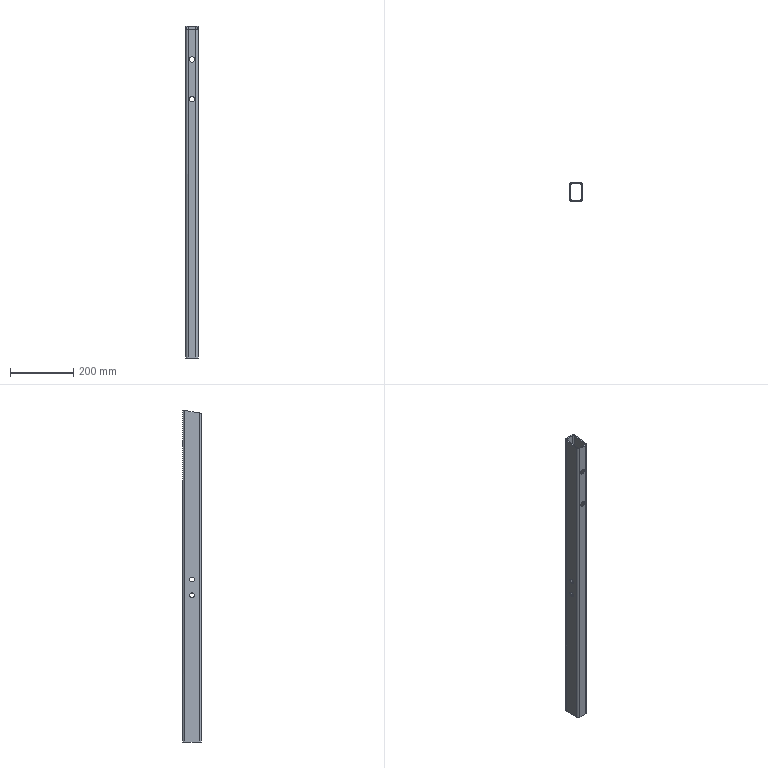Part | SolidWorks | features BaseBody 1 | 1 solid | 34 faces | box 40 x 60 x 1052 mm | volume 553157 mm3 | cylinder 24 | plane 10 | commonest cylinder face diameters 15 x12 17 x8 9 x4
STEP:
#1=CARTESIAN_POINT('',(-17.,7.5,465.));
#2=VERTEX_POINT('',#1);
#3=CARTESIAN_POINT('',(-17.,-7.5,465.));
#4=VERTEX_POINT('',#3);
#5=CARTESIAN_POINT('',(-17.,0.,465.));
#6=DIRECTION('',(-1.,0.,0.));
#7=DIRECTION('',(0.,-1.,0.));
#8=AXIS2_PLACEMENT_3D('',#5,#6,#7);
#9=CIRCLE('',#8,7.5);
#10=EDGE_CURVE('',#2,#4,#9,.T.);
#11=ORIENTED_EDGE('',*,*,#10,.F.);
#12=CARTESIAN_POINT('',(-20.,7.5,465.));
#13=VERTEX_POINT('',#12);
#14=CARTESIAN_POINT('',(1034.474,7.5,465.));
#15=DIRECTION('',(-1.,0.,0.));
#16=VECTOR('',#15,1000.);
#17=LINE('',#14,#16);
#18=EDGE_CURVE('',#2,#13,#17,.T.);
#19=ORIENTED_EDGE('',*,*,#18,.T.);
#20=CARTESIAN_POINT('',(-20.,-7.5,465.));
#21=VERTEX_POINT('',#20);
#22=CARTESIAN_POINT('',(-20.,0.,465.));
#23=DIRECTION('',(1.,0.,0.));
#24=DIRECTION('',(0.,-1.,0.));
#25=AXIS2_PLACEMENT_3D('',#22,#23,#24);
#26=CIRCLE('',#25,7.5);
#27=EDGE_CURVE('',#21,#13,#26,.T.);
#28=ORIENTED_EDGE('',*,*,#27,.F.);
#29=CARTESIAN_POINT('',(1034.474,-7.5,465.));
#30=DIRECTION('',(-1.,0.,0.));
#31=VECTOR('',#30,1000.);
#32=LINE('',#29,#31);
#33=EDGE_CURVE('',#4,#21,#32,.T.);
#34=ORIENTED_EDGE('',*,*,#33,.F.);
#35=EDGE_LOOP('',(#11,#19,#28,#34));
#36=FACE_OUTER_BOUND('',#35,.T.);
#37=CARTESIAN_POINT('',(1034.474,0.,465.));
#38=DIRECTION('',(-1.,0.,0.));
#39=DIRECTION('',(0.,-1.,0.));
#40=AXIS2_PLACEMENT_3D('',#37,#38,#39);
#41=CYLINDRICAL_SURFACE('',#40,7.5);
#42=ADVANCED_FACE('',(#36),#41,.F.);
#43=CARTESIAN_POINT('',(-17.,7.5,515.));
#44=VERTEX_POINT('',#43);
#45=CARTESIAN_POINT('',(-17.,-7.5,515.));
#46=VERTEX_POINT('',#45);
#47=CARTESIAN_POINT('',(-17.,0.,515.));
#48=DIRECTION('',(-1.,0.,0.));
#49=DIRECTION('',(0.,-1.,0.));
#50=AXIS2_PLACEMENT_3D('',#47,#48,#49);
#51=CIRCLE('',#50,7.5);
#52=EDGE_CURVE('',#44,#46,#51,.T.);
#53=ORIENTED_EDGE('',*,*,#52,.F.);
#54=CARTESIAN_POINT('',(-20.,7.5,515.));
#55=VERTEX_POINT('',#54);
#56=CARTESIAN_POINT('',(1034.474,7.5,515.));
#57=DIRECTION('',(-1.,0.,0.));
#58=VECTOR('',#57,1000.);
#59=LINE('',#56,#58);
#60=EDGE_CURVE('',#44,#55,#59,.T.);
#61=ORIENTED_EDGE('',*,*,#60,.T.);
#62=CARTESIAN_POINT('',(-20.,-7.5,515.));
#63=VERTEX_POINT('',#62);
#64=CARTESIAN_POINT('',(-20.,0.,515.));
#65=DIRECTION('',(1.,0.,0.));
#66=DIRECTION('',(0.,-1.,0.));
#67=AXIS2_PLACEMENT_3D('',#64,#65,#66);
#68=CIRCLE('',#67,7.5);
#69=EDGE_CURVE('',#63,#55,#68,.T.);
#70=ORIENTED_EDGE('',*,*,#69,.F.);
#71=CARTESIAN_POINT('',(1034.474,-7.5,515.));
#72=DIRECTION('',(-1.,0.,0.));
#73=VECTOR('',#72,1000.);
#74=LINE('',#71,#73);
#75=EDGE_CURVE('',#46,#63,#74,.T.);
#76=ORIENTED_EDGE('',*,*,#75,.F.);
#77=EDGE_LOOP('',(#53,#61,#70,#76));
#78=FACE_OUTER_BOUND('',#77,.T.);
#79=CARTESIAN_POINT('',(1034.474,0.,515.));
#80=DIRECTION('',(-1.,0.,0.));
#81=DIRECTION('',(0.,-1.,0.));
#82=AXIS2_PLACEMENT_3D('',#79,#80,#81);
#83=CYLINDRICAL_SURFACE('',#82,7.5);
#84=ADVANCED_FACE('',(#78),#83,.F.);
#85=CARTESIAN_POINT('',(0.,-30.,937.5));
#86=VERTEX_POINT('',#85);
#87=CARTESIAN_POINT('',(0.,-30.,954.5));
#88=VERTEX_POINT('',#87);
#89=CARTESIAN_POINT('',(0.,-30.,946.));
#90=DIRECTION('',(0.,1.,0.));
#91=DIRECTION('',(0.,0.,1.));
#92=AXIS2_PLACEMENT_3D('',#89,#90,#91);
#93=CIRCLE('',#92,8.5);
#94=EDGE_CURVE('',#86,#88,#93,.T.);
#95=ORIENTED_EDGE('',*,*,#94,.F.);
#96=CARTESIAN_POINT('',(0.,-27.,937.5));
#97=VERTEX_POINT('',#96);
#98=CARTESIAN_POINT('',(0.,-1024.474,937.5));
#99=DIRECTION('',(0.,1.,0.));
#100=VECTOR('',#99,1000.);
#101=LINE('',#98,#100);
#102=EDGE_CURVE('',#86,#97,#101,.T.);
#103=ORIENTED_EDGE('',*,*,#102,.T.);
#104=CARTESIAN_POINT('',(0.,-27.,954.5));
#105=VERTEX_POINT('',#104);
#106=CARTESIAN_POINT('',(0.,-27.,946.));
#107=DIRECTION('',(0.,1.,0.));
#108=DIRECTION('',(0.,0.,1.));
#109=AXIS2_PLACEMENT_3D('',#106,#107,#108);
#110=CIRCLE('',#109,8.5);
#111=EDGE_CURVE('',#97,#105,#110,.T.);
#112=ORIENTED_EDGE('',*,*,#111,.T.);
#113=CARTESIAN_POINT('',(0.,-1024.474,954.5));
#114=DIRECTION('',(0.,1.,0.));
#115=VECTOR('',#114,1000.);
#116=LINE('',#113,#115);
#117=EDGE_CURVE('',#88,#105,#116,.T.);
#118=ORIENTED_EDGE('',*,*,#117,.F.);
#119=EDGE_LOOP('',(#95,#103,#112,#118));
#120=FACE_OUTER_BOUND('',#119,.T.);
#121=CARTESIAN_POINT('',(0.,-1024.474,946.));
#122=DIRECTION('',(0.,1.,0.));
#123=DIRECTION('',(0.,0.,1.));
#124=AXIS2_PLACEMENT_3D('',#121,#122,#123);
#125=CYLINDRICAL_SURFACE('',#124,8.5);
#126=ADVANCED_FACE('',(#120),#125,.F.);
#127=CARTESIAN_POINT('',(0.,-30.,811.5));
#128=VERTEX_POINT('',#127);
#129=CARTESIAN_POINT('',(0.,-30.,828.5));
#130=VERTEX_POINT('',#129);
#131=CARTESIAN_POINT('',(0.,-30.,820.));
#132=DIRECTION('',(0.,1.,0.));
#133=DIRECTION('',(0.,0.,1.));
#134=AXIS2_PLACEMENT_3D('',#131,#132,#133);
#135=CIRCLE('',#134,8.5);
#136=EDGE_CURVE('',#128,#130,#135,.T.);
#137=ORIENTED_EDGE('',*,*,#136,.F.);
#138=CARTESIAN_POINT('',(0.,-27.,811.5));
#139=VERTEX_POINT('',#138);
#140=CARTESIAN_POINT('',(0.,-1024.474,811.5));
#141=DIRECTION('',(0.,1.,0.));
#142=VECTOR('',#141,1000.);
#143=LINE('',#140,#142);
#144=EDGE_CURVE('',#128,#139,#143,.T.);
#145=ORIENTED_EDGE('',*,*,#144,.T.);
#146=CARTESIAN_POINT('',(0.,-27.,828.5));
#147=VERTEX_POINT('',#146);
#148=CARTESIAN_POINT('',(0.,-27.,820.));
#149=DIRECTION('',(0.,1.,0.));
#150=DIRECTION('',(0.,0.,1.));
#151=AXIS2_PLACEMENT_3D('',#148,#149,#150);
#152=CIRCLE('',#151,8.5);
#153=EDGE_CURVE('',#139,#147,#152,.T.);
#154=ORIENTED_EDGE('',*,*,#153,.T.);
#155=CARTESIAN_POINT('',(0.,-1024.474,828.5));
#156=DIRECTION('',(0.,1.,0.));
#157=VECTOR('',#156,1000.);
#158=LINE('',#155,#157);
#159=EDGE_CURVE('',#130,#147,#158,.T.);
#160=ORIENTED_EDGE('',*,*,#159,.F.);
#161=EDGE_LOOP('',(#137,#145,#154,#160));
#162=FACE_OUTER_BOUND('',#161,.T.);
#163=CARTESIAN_POINT('',(0.,-1024.474,820.));
#164=DIRECTION('',(0.,1.,0.));
#165=DIRECTION('',(0.,0.,1.));
#166=AXIS2_PLACEMENT_3D('',#163,#164,#165);
#167=CYLINDRICAL_SURFACE('',#166,8.5);
#168=ADVANCED_FACE('',(#162),#167,.F.);
#169=CARTESIAN_POINT('',(0.,27.,954.5));
#170=VERTEX_POINT('',#169);
#171=CARTESIAN_POINT('',(0.,27.,937.5));
#172=VERTEX_POINT('',#171);
#173=CARTESIAN_POINT('',(0.,27.,946.));
#174=DIRECTION('',(0.,-1.,0.));
#175=DIRECTION('',(0.,0.,1.));
#176=AXIS2_PLACEMENT_3D('',#173,#174,#175);
#177=CIRCLE('',#176,8.5);
#178=EDGE_CURVE('',#170,#172,#177,.T.);
#179=ORIENTED_EDGE('',*,*,#178,.T.);
#180=CARTESIAN_POINT('',(0.,30.,937.5));
#181=VERTEX_POINT('',#180);
#182=CARTESIAN_POINT('',(0.,-1024.474,937.5));
#183=DIRECTION('',(0.,1.,0.));
#184=VECTOR('',#183,1000.);
#185=LINE('',#182,#184);
#186=EDGE_CURVE('',#172,#181,#185,.T.);
#187=ORIENTED_EDGE('',*,*,#186,.T.);
#188=CARTESIAN_POINT('',(0.,30.,954.5));
#189=VERTEX_POINT('',#188);
#190=CARTESIAN_POINT('',(0.,30.,946.));
#191=DIRECTION('',(0.,-1.,0.));
#192=DIRECTION('',(0.,0.,1.));
#193=AXIS2_PLACEMENT_3D('',#190,#191,#192);
#194=CIRCLE('',#193,8.5);
#195=EDGE_CURVE('',#189,#181,#194,.T.);
#196=ORIENTED_EDGE('',*,*,#195,.F.);
#197=CARTESIAN_POINT('',(0.,-1024.474,954.5));
#198=DIRECTION('',(0.,1.,0.));
#199=VECTOR('',#198,1000.);
#200=LINE('',#197,#199);
#201=EDGE_CURVE('',#170,#189,#200,.T.);
#202=ORIENTED_EDGE('',*,*,#201,.F.);
#203=EDGE_LOOP('',(#179,#187,#196,#202));
#204=FACE_OUTER_BOUND('',#203,.T.);
#205=CARTESIAN_POINT('',(0.,-1024.474,946.));
#206=DIRECTION('',(0.,1.,0.));
#207=DIRECTION('',(0.,0.,1.));
#208=AXIS2_PLACEMENT_3D('',#205,#206,#207);
#209=CYLINDRICAL_SURFACE('',#208,8.5);
#210=ADVANCED_FACE('',(#204),#209,.F.);
#211=CARTESIAN_POINT('',(0.,27.,828.5));
#212=VERTEX_POINT('',#211);
#213=CARTESIAN_POINT('',(0.,27.,811.5));
#214=VERTEX_POINT('',#213);
#215=CARTESIAN_POINT('',(0.,27.,820.));
#216=DIRECTION('',(0.,-1.,0.));
#217=DIRECTION('',(0.,0.,1.));
#218=AXIS2_PLACEMENT_3D('',#215,#216,#217);
#219=CIRCLE('',#218,8.5);
#220=EDGE_CURVE('',#212,#214,#219,.T.);
#221=ORIENTED_EDGE('',*,*,#220,.T.);
#222=CARTESIAN_POINT('',(0.,30.,811.5));
#223=VERTEX_POINT('',#222);
#224=CARTESIAN_POINT('',(0.,-1024.474,811.5));
#225=DIRECTION('',(0.,1.,0.));
#226=VECTOR('',#225,1000.);
#227=LINE('',#224,#226);
#228=EDGE_CURVE('',#214,#223,#227,.T.);
#229=ORIENTED_EDGE('',*,*,#228,.T.);
#230=CARTESIAN_POINT('',(0.,30.,828.5));
#231=VERTEX_POINT('',#230);
#232=CARTESIAN_POINT('',(0.,30.,820.));
#233=DIRECTION('',(0.,-1.,0.));
#234=DIRECTION('',(0.,0.,1.));
#235=AXIS2_PLACEMENT_3D('',#232,#233,#234);
#236=CIRCLE('',#235,8.5);
#237=EDGE_CURVE('',#231,#223,#236,.T.);
#238=ORIENTED_EDGE('',*,*,#237,.F.);
#239=CARTESIAN_POINT('',(0.,-1024.474,828.5));
#240=DIRECTION('',(0.,1.,0.));
#241=VECTOR('',#240,1000.);
#242=LINE('',#239,#241);
#243=EDGE_CURVE('',#212,#231,#242,.T.);
#244=ORIENTED_EDGE('',*,*,#243,.F.);
#245=EDGE_LOOP('',(#221,#229,#238,#244));
#246=FACE_OUTER_BOUND('',#245,.T.);
#247=CARTESIAN_POINT('',(0.,-1024.474,820.));
#248=DIRECTION('',(0.,1.,0.));
#249=DIRECTION('',(0.,0.,1.));
#250=AXIS2_PLACEMENT_3D('',#247,#248,#249);
#251=CYLINDRICAL_SURFACE('',#250,8.5);
#252=ADVANCED_FACE('',(#246),#251,.F.);
#253=CARTESIAN_POINT('',(20.,7.5,465.));
#254=VERTEX_POINT('',#253);
#255=CARTESIAN_POINT('',(20.,-7.5,465.));
#256=VERTEX_POINT('',#255);
#257=CARTESIAN_POINT('',(20.,0.,465.));
#258=DIRECTION('',(-1.,0.,0.));
#259=DIRECTION('',(0.,-1.,0.));
#260=AXIS2_PLACEMENT_3D('',#257,#258,#259);
#261=CIRCLE('',#260,7.5);
#262=EDGE_CURVE('',#254,#256,#261,.T.);
#263=ORIENTED_EDGE('',*,*,#262,.F.);
#264=CARTESIAN_POINT('',(17.,7.5,465.));
#265=VERTEX_POINT('',#264);
#266=CARTESIAN_POINT('',(1034.474,7.5,465.));
#267=DIRECTION('',(-1.,0.,0.));
#268=VECTOR('',#267,1000.);
#269=LINE('',#266,#268);
#270=EDGE_CURVE('',#254,#265,#269,.T.);
#271=ORIENTED_EDGE('',*,*,#270,.T.);
#272=CARTESIAN_POINT('',(17.,-7.5,465.));
#273=VERTEX_POINT('',#272);
#274=CARTESIAN_POINT('',(17.,0.,465.));
#275=DIRECTION('',(-1.,0.,0.));
#276=DIRECTION('',(0.,-1.,0.));
#277=AXIS2_PLACEMENT_3D('',#274,#275,#276);
#278=CIRCLE('',#277,7.5);
#279=EDGE_CURVE('',#265,#273,#278,.T.);
#280=ORIENTED_EDGE('',*,*,#279,.T.);
#281=CARTESIAN_POINT('',(1034.474,-7.5,465.));
#282=DIRECTION('',(-1.,0.,0.));
#283=VECTOR('',#282,1000.);
#284=LINE('',#281,#283);
#285=EDGE_CURVE('',#256,#273,#284,.T.);
#286=ORIENTED_EDGE('',*,*,#285,.F.);
#287=EDGE_LOOP('',(#263,#271,#280,#286));
#288=FACE_OUTER_BOUND('',#287,.T.);
#289=CARTESIAN_POINT('',(1034.474,0.,465.));
#290=DIRECTION('',(-1.,0.,0.));
#291=DIRECTION('',(0.,-1.,0.));
#292=AXIS2_PLACEMENT_3D('',#289,#290,#291);
#293=CYLINDRICAL_SURFACE('',#292,7.5);
#294=ADVANCED_FACE('',(#288),#293,.F.);
#295=CARTESIAN_POINT('',(20.,7.5,515.));
#296=VERTEX_POINT('',#295);
#297=CARTESIAN_POINT('',(20.,-7.5,515.));
#298=VERTEX_POINT('',#297);
#299=CARTESIAN_POINT('',(20.,0.,515.));
#300=DIRECTION('',(-1.,0.,0.));
#301=DIRECTION('',(0.,-1.,0.));
#302=AXIS2_PLACEMENT_3D('',#299,#300,#301);
#303=CIRCLE('',#302,7.5);
#304=EDGE_CURVE('',#296,#298,#303,.T.);
#305=ORIENTED_EDGE('',*,*,#304,.F.);
#306=CARTESIAN_POINT('',(17.,7.5,515.));
#307=VERTEX_POINT('',#306);
#308=CARTESIAN_POINT('',(1034.474,7.5,515.));
#309=DIRECTION('',(-1.,0.,0.));
#310=VECTOR('',#309,1000.);
#311=LINE('',#308,#310);
#312=EDGE_CURVE('',#296,#307,#311,.T.);
#313=ORIENTED_EDGE('',*,*,#312,.T.);
#314=CARTESIAN_POINT('',(17.,-7.5,515.));
#315=VERTEX_POINT('',#314);
#316=CARTESIAN_POINT('',(17.,0.,515.));
#317=DIRECTION('',(-1.,0.,0.));
#318=DIRECTION('',(0.,-1.,0.));
#319=AXIS2_PLACEMENT_3D('',#316,#317,#318);
#320=CIRCLE('',#319,7.5);
#321=EDGE_CURVE('',#307,#315,#320,.T.);
#322=ORIENTED_EDGE('',*,*,#321,.T.);
#323=CARTESIAN_POINT('',(1034.474,-7.5,515.));
#324=DIRECTION('',(-1.,0.,0.));
#325=VECTOR('',#324,1000.);
#326=LINE('',#323,#325);
#327=EDGE_CURVE('',#298,#315,#326,.T.);
#328=ORIENTED_EDGE('',*,*,#327,.F.);
#329=EDGE_LOOP('',(#305,#313,#322,#328));
#330=FACE_OUTER_BOUND('',#329,.T.);
#331=CARTESIAN_POINT('',(1034.474,0.,515.));
#332=DIRECTION('',(-1.,0.,0.));
#333=DIRECTION('',(0.,-1.,0.));
#334=AXIS2_PLACEMENT_3D('',#331,#332,#333);
#335=CYLINDRICAL_SURFACE('',#334,7.5);
#336=ADVANCED_FACE('',(#330),#335,.F.);
#337=ORIENTED_EDGE('',*,*,#27,.T.);
#338=CARTESIAN_POINT('',(-20.,0.,465.));
#339=DIRECTION('',(1.,0.,0.));
#340=DIRECTION('',(0.,-1.,0.));
#341=AXIS2_PLACEMENT_3D('',#338,#339,#340);
#342=CIRCLE('',#341,7.5);
#343=EDGE_CURVE('',#13,#21,#342,.T.);
#344=ORIENTED_EDGE('',*,*,#343,.T.);
#345=EDGE_LOOP('',(#337,#344));
#346=FACE_BOUND('',#345,.T.);
#347=ORIENTED_EDGE('',*,*,#69,.T.);
#348=CARTESIAN_POINT('',(-20.,0.,515.));
#349=DIRECTION('',(1.,0.,0.));
#350=DIRECTION('',(0.,-1.,0.));
#351=AXIS2_PLACEMENT_3D('',#348,#349,#350);
#352=CIRCLE('',#351,7.5);
#353=EDGE_CURVE('',#55,#63,#352,.T.);
#354=ORIENTED_EDGE('',*,*,#353,.T.);
#355=EDGE_LOOP('',(#347,#354));
#356=FACE_BOUND('',#355,.T.);
#357=CARTESIAN_POINT('',(-20.,22.5,0.));
#358=VERTEX_POINT('',#357);
#359=CARTESIAN_POINT('',(-20.,-22.5,0.));
#360=VERTEX_POINT('',#359);
#361=CARTESIAN_POINT('',(-20.,-22.5,0.));
#362=DIRECTION('',(0.,-1.,0.));
#363=VECTOR('',#362,1000.);
#364=LINE('',#361,#363);
#365=EDGE_CURVE('',#358,#360,#364,.T.);
#366=ORIENTED_EDGE('',*,*,#365,.T.);
#367=CARTESIAN_POINT('',(-20.,-22.5,1042.748));
#368=VERTEX_POINT('',#367);
#369=CARTESIAN_POINT('',(-20.,-22.5,0.));
#370=DIRECTION('',(0.,0.,1.));
#371=VECTOR('',#370,1000.);
#372=LINE('',#369,#371);
#373=EDGE_CURVE('',#360,#368,#372,.T.);
#374=ORIENTED_EDGE('',*,*,#373,.T.);
#375=CARTESIAN_POINT('',(-20.,22.5,1050.683));
#376=VERTEX_POINT('',#375);
#377=CARTESIAN_POINT('',(-20.,-22.5,1042.748));
#378=DIRECTION('',(0.,0.9848,0.1736));
#379=VECTOR('',#378,1000.);
#380=LINE('',#377,#379);
#381=EDGE_CURVE('',#368,#376,#380,.T.);
#382=ORIENTED_EDGE('',*,*,#381,.T.);
#383=CARTESIAN_POINT('',(-20.,22.5,0.));
#384=DIRECTION('',(0.,0.,-1.));
#385=VECTOR('',#384,1000.);
#386=LINE('',#383,#385);
#387=EDGE_CURVE('',#376,#358,#386,.T.);
#388=ORIENTED_EDGE('',*,*,#387,.T.);
#389=EDGE_LOOP('',(#366,#374,#382,#388));
#390=FACE_OUTER_BOUND('',#389,.T.);
#391=CARTESIAN_POINT('',(-20.,-22.5,0.));
#392=DIRECTION('',(-1.,0.,0.));
#393=DIRECTION('',(0.,-1.,0.));
#394=AXIS2_PLACEMENT_3D('',#391,#392,#393);
#395=PLANE('',#394);
#396=ADVANCED_FACE('',(#346,#356,#390),#395,.T.);
#397=ORIENTED_EDGE('',*,*,#18,.F.);
#398=CARTESIAN_POINT('',(-17.,0.,465.));
#399=DIRECTION('',(-1.,0.,0.));
#400=DIRECTION('',(0.,-1.,0.));
#401=AXIS2_PLACEMENT_3D('',#398,#399,#400);
#402=CIRCLE('',#401,7.5);
#403=EDGE_CURVE('',#4,#2,#402,.T.);
#404=ORIENTED_EDGE('',*,*,#403,.F.);
#405=ORIENTED_EDGE('',*,*,#33,.T.);
#406=ORIENTED_EDGE('',*,*,#343,.F.);
#407=EDGE_LOOP('',(#397,#404,#405,#406));
#408=FACE_OUTER_BOUND('',#407,.T.);
#409=CARTESIAN_POINT('',(1034.474,0.,465.));
#410=DIRECTION('',(-1.,0.,0.));
#411=DIRECTION('',(0.,-1.,0.));
#412=AXIS2_PLACEMENT_3D('',#409,#410,#411);
#413=CYLINDRICAL_SURFACE('',#412,7.5);
#414=ADVANCED_FACE('',(#408),#413,.F.);
#415=ORIENTED_EDGE('',*,*,#60,.F.);
#416=CARTESIAN_POINT('',(-17.,0.,515.));
#417=DIRECTION('',(-1.,0.,0.));
#418=DIRECTION('',(0.,-1.,0.));
#419=AXIS2_PLACEMENT_3D('',#416,#417,#418);
#420=CIRCLE('',#419,7.5);
#421=EDGE_CURVE('',#46,#44,#420,.T.);
#422=ORIENTED_EDGE('',*,*,#421,.F.);
#423=ORIENTED_EDGE('',*,*,#75,.T.);
#424=ORIENTED_EDGE('',*,*,#353,.F.);
#425=EDGE_LOOP('',(#415,#422,#423,#424));
#426=FACE_OUTER_BOUND('',#425,.T.);
#427=CARTESIAN_POINT('',(1034.474,0.,515.));
#428=DIRECTION('',(-1.,0.,0.));
#429=DIRECTION('',(0.,-1.,0.));
#430=AXIS2_PLACEMENT_3D('',#427,#428,#429);
#431=CYLINDRICAL_SURFACE('',#430,7.5);
#432=ADVANCED_FACE('',(#426),#431,.F.);
#433=CARTESIAN_POINT('',(-12.5,-30.,0.));
#434=VERTEX_POINT('',#433);
#435=CARTESIAN_POINT('',(-12.5,-22.5,0.));
#436=DIRECTION('',(0.,0.,1.));
#437=DIRECTION('',(1.,0.,0.));
#438=AXIS2_PLACEMENT_3D('',#435,#436,#437);
#439=CIRCLE('',#438,7.5);
#440=EDGE_CURVE('',#360,#434,#439,.T.);
#441=ORIENTED_EDGE('',*,*,#440,.T.);
#442=CARTESIAN_POINT('',(-12.5,-30.,1041.426));
#443=VERTEX_POINT('',#442);
#444=CARTESIAN_POINT('',(-12.5,-30.,0.));
#445=DIRECTION('',(0.,0.,1.));
#446=VECTOR('',#445,1000.);
#447=LINE('',#444,#446);
#448=EDGE_CURVE('',#434,#443,#447,.T.);
#449=ORIENTED_EDGE('',*,*,#448,.T.);
#450=CARTESIAN_POINT('',(-12.5,-30.,1041.426));
#451=CARTESIAN_POINT('',(-16.893,-30.,1041.426));
#452=CARTESIAN_POINT('',(-20.,-26.893,1041.974));
#453=CARTESIAN_POINT('',(-20.,-22.5,1042.748));
#454=(BOUNDED_CURVE()B_SPLINE_CURVE(3,(#450,#451,#452,#453),.UNSPECIFIED.,.F.,.T.)B_SPLINE_CURVE_WITH_KNOTS((4,4),(3.142,4.712),.UNSPECIFIED.)CURVE()GEOMETRIC_REPRESENTATION_ITEM()RATIONAL_B_SPLINE_CURVE((1.,0.8047,0.8047,1.))REPRESENTATION_ITEM(''));
#455=EDGE_CURVE('',#443,#368,#454,.T.);
#456=ORIENTED_EDGE('',*,*,#455,.T.);
#457=ORIENTED_EDGE('',*,*,#373,.F.);
#458=EDGE_LOOP('',(#441,#449,#456,#457));
#459=FACE_OUTER_BOUND('',#458,.T.);
#460=CARTESIAN_POINT('',(-12.5,-22.5,0.));
#461=DIRECTION('',(0.,0.,1.));
#462=DIRECTION('',(1.,0.,0.));
#463=AXIS2_PLACEMENT_3D('',#460,#461,#462);
#464=CYLINDRICAL_SURFACE('',#463,7.5);
#465=ADVANCED_FACE('',(#459),#464,.T.);
#466=CARTESIAN_POINT('',(-17.,22.5,0.));
#467=VERTEX_POINT('',#466);
#468=CARTESIAN_POINT('',(-12.5,27.,0.));
#469=VERTEX_POINT('',#468);
#470=CARTESIAN_POINT('',(-12.5,22.5,0.));
#471=DIRECTION('',(0.,0.,-1.));
#472=DIRECTION('',(1.,0.,0.));
#473=AXIS2_PLACEMENT_3D('',#470,#471,#472);
#474=CIRCLE('',#473,4.5);
#475=EDGE_CURVE('',#467,#469,#474,.T.);
#476=ORIENTED_EDGE('',*,*,#475,.F.);
#477=CARTESIAN_POINT('',(-17.,-22.5,0.));
#478=VERTEX_POINT('',#477);
#479=CARTESIAN_POINT('',(-17.,0.,0.));
#480=DIRECTION('',(0.,1.,0.));
#481=VECTOR('',#480,1000.);
#482=LINE('',#479,#481);
#483=EDGE_CURVE('',#478,#467,#482,.T.);
#484=ORIENTED_EDGE('',*,*,#483,.F.);
#485=CARTESIAN_POINT('',(-12.5,-27.,0.));
#486=VERTEX_POINT('',#485);
#487=CARTESIAN_POINT('',(-12.5,-22.5,0.));
#488=DIRECTION('',(0.,0.,-1.));
#489=DIRECTION('',(1.,0.,0.));
#490=AXIS2_PLACEMENT_3D('',#487,#488,#489);
#491=CIRCLE('',#490,4.5);
#492=EDGE_CURVE('',#486,#478,#491,.T.);
#493=ORIENTED_EDGE('',*,*,#492,.F.);
#494=CARTESIAN_POINT('',(12.5,-27.,0.));
#495=VERTEX_POINT('',#494);
#496=CARTESIAN_POINT('',(0.,-27.,0.));
#497=DIRECTION('',(-1.,0.,0.));
#498=VECTOR('',#497,1000.);
#499=LINE('',#496,#498);
#500=EDGE_CURVE('',#495,#486,#499,.T.);
#501=ORIENTED_EDGE('',*,*,#500,.F.);
#502=CARTESIAN_POINT('',(17.,-22.5,0.));
#503=VERTEX_POINT('',#502);
#504=CARTESIAN_POINT('',(12.5,-22.5,0.));
#505=DIRECTION('',(0.,0.,-1.));
#506=DIRECTION('',(1.,0.,0.));
#507=AXIS2_PLACEMENT_3D('',#504,#505,#506);
#508=CIRCLE('',#507,4.5);
#509=EDGE_CURVE('',#503,#495,#508,.T.);
#510=ORIENTED_EDGE('',*,*,#509,.F.);
#511=CARTESIAN_POINT('',(17.,22.5,0.));
#512=VERTEX_POINT('',#511);
#513=CARTESIAN_POINT('',(17.,0.,0.));
#514=DIRECTION('',(0.,-1.,0.));
#515=VECTOR('',#514,1000.);
#516=LINE('',#513,#515);
#517=EDGE_CURVE('',#512,#503,#516,.T.);
#518=ORIENTED_EDGE('',*,*,#517,.F.);
#519=CARTESIAN_POINT('',(12.5,27.,0.));
#520=VERTEX_POINT('',#519);
#521=CARTESIAN_POINT('',(12.5,22.5,0.));
#522=DIRECTION('',(0.,0.,-1.));
#523=DIRECTION('',(1.,0.,0.));
#524=AXIS2_PLACEMENT_3D('',#521,#522,#523);
#525=CIRCLE('',#524,4.5);
#526=EDGE_CURVE('',#520,#512,#525,.T.);
#527=ORIENTED_EDGE('',*,*,#526,.F.);
#528=CARTESIAN_POINT('',(0.,27.,0.));
#529=DIRECTION('',(1.,0.,0.));
#530=VECTOR('',#529,1000.);
#531=LINE('',#528,#530);
#532=EDGE_CURVE('',#469,#520,#531,.T.);
#533=ORIENTED_EDGE('',*,*,#532,.F.);
#534=EDGE_LOOP('',(#476,#484,#493,#501,#510,#518,#527,#533));
#535=FACE_BOUND('',#534,.T.);
#536=CARTESIAN_POINT('',(-12.5,30.,0.));
#537=VERTEX_POINT('',#536);
#538=CARTESIAN_POINT('',(-12.5,22.5,0.));
#539=DIRECTION('',(0.,0.,1.));
#540=DIRECTION('',(1.,0.,0.));
#541=AXIS2_PLACEMENT_3D('',#538,#539,#540);
#542=CIRCLE('',#541,7.5);
#543=EDGE_CURVE('',#537,#358,#542,.T.);
#544=ORIENTED_EDGE('',*,*,#543,.F.);
#545=CARTESIAN_POINT('',(12.5,30.,0.));
#546=VERTEX_POINT('',#545);
#547=CARTESIAN_POINT('',(0.,30.,0.));
#548=DIRECTION('',(-1.,0.,0.));
#549=VECTOR('',#548,1000.);
#550=LINE('',#547,#549);
#551=EDGE_CURVE('',#546,#537,#550,.T.);
#552=ORIENTED_EDGE('',*,*,#551,.F.);
#553=CARTESIAN_POINT('',(20.,22.5,0.));
#554=VERTEX_POINT('',#553);
#555=CARTESIAN_POINT('',(12.5,22.5,0.));
#556=DIRECTION('',(0.,0.,1.));
#557=DIRECTION('',(1.,0.,0.));
#558=AXIS2_PLACEMENT_3D('',#555,#556,#557);
#559=CIRCLE('',#558,7.5);
#560=EDGE_CURVE('',#554,#546,#559,.T.);
#561=ORIENTED_EDGE('',*,*,#560,.F.);
#562=CARTESIAN_POINT('',(20.,-22.5,0.));
#563=VERTEX_POINT('',#562);
#564=CARTESIAN_POINT('',(20.,0.,0.));
#565=DIRECTION('',(0.,1.,0.));
#566=VECTOR('',#565,1000.);
#567=LINE('',#564,#566);
#568=EDGE_CURVE('',#563,#554,#567,.T.);
#569=ORIENTED_EDGE('',*,*,#568,.F.);
#570=CARTESIAN_POINT('',(12.5,-30.,0.));
#571=VERTEX_POINT('',#570);
#572=CARTESIAN_POINT('',(12.5,-22.5,0.));
#573=DIRECTION('',(0.,0.,1.));
#574=DIRECTION('',(1.,0.,0.));
#575=AXIS2_PLACEMENT_3D('',#572,#573,#574);
#576=CIRCLE('',#575,7.5);
#577=EDGE_CURVE('',#571,#563,#576,.T.);
#578=ORIENTED_EDGE('',*,*,#577,.F.);
#579=CARTESIAN_POINT('',(0.,-30.,0.));
#580=DIRECTION('',(1.,0.,0.));
#581=VECTOR('',#580,1000.);
#582=LINE('',#579,#581);
#583=EDGE_CURVE('',#434,#571,#582,.T.);
#584=ORIENTED_EDGE('',*,*,#583,.F.);
#585=ORIENTED_EDGE('',*,*,#440,.F.);
#586=ORIENTED_EDGE('',*,*,#365,.F.);
#587=EDGE_LOOP('',(#544,#552,#561,#569,#578,#584,#585,#586));
#588=FACE_OUTER_BOUND('',#587,.T.);
#589=CARTESIAN_POINT('',(0.,0.,0.));
#590=DIRECTION('',(0.,0.,1.));
#591=DIRECTION('',(1.,0.,0.));
#592=AXIS2_PLACEMENT_3D('',#589,#590,#591);
#593=PLANE('',#592);
#594=ADVANCED_FACE('',(#535,#588),#593,.F.);
#595=ORIENTED_EDGE('',*,*,#543,.T.);
#596=ORIENTED_EDGE('',*,*,#387,.F.);
#597=CARTESIAN_POINT('',(-12.5,30.,1052.005));
#598=VERTEX_POINT('',#597);
#599=CARTESIAN_POINT('',(-20.,22.5,1050.683));
#600=CARTESIAN_POINT('',(-20.,26.893,1051.458));
#601=CARTESIAN_POINT('',(-16.893,30.,1052.005));
#602=CARTESIAN_POINT('',(-12.5,30.,1052.005));
#603=(BOUNDED_CURVE()B_SPLINE_CURVE(3,(#599,#600,#601,#602),.UNSPECIFIED.,.F.,.F.)B_SPLINE_CURVE_WITH_KNOTS((4,4),(4.712,6.283),.UNSPECIFIED.)CURVE()GEOMETRIC_REPRESENTATION_ITEM()RATIONAL_B_SPLINE_CURVE((1.,0.8047,0.8047,1.))REPRESENTATION_ITEM(''));
#604=EDGE_CURVE('',#376,#598,#603,.T.);
#605=ORIENTED_EDGE('',*,*,#604,.T.);
#606=CARTESIAN_POINT('',(-12.5,30.,0.));
#607=DIRECTION('',(0.,0.,-1.));
#608=VECTOR('',#607,1000.);
#609=LINE('',#606,#608);
#610=EDGE_CURVE('',#598,#537,#609,.T.);
#611=ORIENTED_EDGE('',*,*,#610,.T.);
#612=EDGE_LOOP('',(#595,#596,#605,#611));
#613=FACE_OUTER_BOUND('',#612,.T.);
#614=CARTESIAN_POINT('',(-12.5,22.5,0.));
#615=DIRECTION('',(0.,0.,1.));
#616=DIRECTION('',(1.,0.,0.));
#617=AXIS2_PLACEMENT_3D('',#614,#615,#616);
#618=CYLINDRICAL_SURFACE('',#617,7.5);
#619=ADVANCED_FACE('',(#613),#618,.T.);
#620=CARTESIAN_POINT('',(-17.,-22.5,1042.748));
#621=VERTEX_POINT('',#620);
#622=CARTESIAN_POINT('',(-12.5,-27.,1041.955));
#623=VERTEX_POINT('',#622);
#624=CARTESIAN_POINT('',(-17.,-22.5,1042.748));
#625=CARTESIAN_POINT('',(-17.,-25.136,1042.283));
#626=CARTESIAN_POINT('',(-15.136,-27.,1041.955));
#627=CARTESIAN_POINT('',(-12.5,-27.,1041.955));
#628=(BOUNDED_CURVE()B_SPLINE_CURVE(3,(#624,#625,#626,#627),.UNSPECIFIED.,.F.,.F.)B_SPLINE_CURVE_WITH_KNOTS((4,4),(1.571,3.142),.UNSPECIFIED.)CURVE()GEOMETRIC_REPRESENTATION_ITEM()RATIONAL_B_SPLINE_CURVE((1.,0.8047,0.8047,1.))REPRESENTATION_ITEM(''));
#629=EDGE_CURVE('',#621,#623,#628,.T.);
#630=ORIENTED_EDGE('',*,*,#629,.F.);
#631=CARTESIAN_POINT('',(-17.,22.5,1050.683));
#632=VERTEX_POINT('',#631);
#633=CARTESIAN_POINT('',(-17.,-178.999,1015.153));
#634=DIRECTION('',(0.,-0.9848,-0.1736));
#635=VECTOR('',#634,1000.);
#636=LINE('',#633,#635);
#637=EDGE_CURVE('',#632,#621,#636,.T.);
#638=ORIENTED_EDGE('',*,*,#637,.F.);
#639=CARTESIAN_POINT('',(-12.5,27.,1051.476));
#640=VERTEX_POINT('',#639);
#641=CARTESIAN_POINT('',(-12.5,27.,1051.476));
#642=CARTESIAN_POINT('',(-15.136,27.,1051.476));
#643=CARTESIAN_POINT('',(-17.,25.136,1051.148));
#644=CARTESIAN_POINT('',(-17.,22.5,1050.683));
#645=(BOUNDED_CURVE()B_SPLINE_CURVE(3,(#641,#642,#643,#644),.UNSPECIFIED.,.F.,.F.)B_SPLINE_CURVE_WITH_KNOTS((4,4),(0.,1.571),.UNSPECIFIED.)CURVE()GEOMETRIC_REPRESENTATION_ITEM()RATIONAL_B_SPLINE_CURVE((1.,0.8047,0.8047,1.))REPRESENTATION_ITEM(''));
#646=EDGE_CURVE('',#640,#632,#645,.T.);
#647=ORIENTED_EDGE('',*,*,#646,.F.);
#648=CARTESIAN_POINT('',(12.5,27.,1051.476));
#649=VERTEX_POINT('',#648);
#650=CARTESIAN_POINT('',(0.,27.,1051.476));
#651=DIRECTION('',(-1.,0.,0.));
#652=VECTOR('',#651,1000.);
#653=LINE('',#650,#652);
#654=EDGE_CURVE('',#649,#640,#653,.T.);
#655=ORIENTED_EDGE('',*,*,#654,.F.);
#656=CARTESIAN_POINT('',(17.,22.5,1050.683));
#657=VERTEX_POINT('',#656);
#658=CARTESIAN_POINT('',(17.,22.5,1050.683));
#659=CARTESIAN_POINT('',(17.,25.136,1051.148));
#660=CARTESIAN_POINT('',(15.136,27.,1051.476));
#661=CARTESIAN_POINT('',(12.5,27.,1051.476));
#662=(BOUNDED_CURVE()B_SPLINE_CURVE(3,(#658,#659,#660,#661),.UNSPECIFIED.,.F.,.F.)B_SPLINE_CURVE_WITH_KNOTS((4,4),(4.712,6.283),.UNSPECIFIED.)CURVE()GEOMETRIC_REPRESENTATION_ITEM()RATIONAL_B_SPLINE_CURVE((1.,0.8047,0.8047,1.))REPRESENTATION_ITEM(''));
#663=EDGE_CURVE('',#657,#649,#662,.T.);
#664=ORIENTED_EDGE('',*,*,#663,.F.);
#665=CARTESIAN_POINT('',(17.,-22.5,1042.748));
#666=VERTEX_POINT('',#665);
#667=CARTESIAN_POINT('',(17.,-178.999,1015.153));
#668=DIRECTION('',(0.,0.9848,0.1736));
#669=VECTOR('',#668,1000.);
#670=LINE('',#667,#669);
#671=EDGE_CURVE('',#666,#657,#670,.T.);
#672=ORIENTED_EDGE('',*,*,#671,.F.);
#673=CARTESIAN_POINT('',(12.5,-27.,1041.955));
#674=VERTEX_POINT('',#673);
#675=CARTESIAN_POINT('',(12.5,-27.,1041.955));
#676=CARTESIAN_POINT('',(15.136,-27.,1041.955));
#677=CARTESIAN_POINT('',(17.,-25.136,1042.283));
#678=CARTESIAN_POINT('',(17.,-22.5,1042.748));
#679=(BOUNDED_CURVE()B_SPLINE_CURVE(3,(#675,#676,#677,#678),.UNSPECIFIED.,.F.,.F.)B_SPLINE_CURVE_WITH_KNOTS((4,4),(3.142,4.712),.UNSPECIFIED.)CURVE()GEOMETRIC_REPRESENTATION_ITEM()RATIONAL_B_SPLINE_CURVE((1.,0.8047,0.8047,1.))REPRESENTATION_ITEM(''));
#680=EDGE_CURVE('',#674,#666,#679,.T.);
#681=ORIENTED_EDGE('',*,*,#680,.F.);
#682=CARTESIAN_POINT('',(0.,-27.,1041.955));
#683=DIRECTION('',(1.,0.,0.));
#684=VECTOR('',#683,1000.);
#685=LINE('',#682,#684);
#686=EDGE_CURVE('',#623,#674,#685,.T.);
#687=ORIENTED_EDGE('',*,*,#686,.F.);
#688=EDGE_LOOP('',(#630,#638,#647,#655,#664,#672,#681,#687));
#689=FACE_BOUND('',#688,.T.);
#690=CARTESIAN_POINT('',(12.5,30.,1052.005));
#691=VERTEX_POINT('',#690);
#692=CARTESIAN_POINT('',(20.,22.5,1050.683));
#693=VERTEX_POINT('',#692);
#694=CARTESIAN_POINT('',(12.5,30.,1052.005));
#695=CARTESIAN_POINT('',(16.893,30.,1052.005));
#696=CARTESIAN_POINT('',(20.,26.893,1051.458));
#697=CARTESIAN_POINT('',(20.,22.5,1050.683));
#698=(BOUNDED_CURVE()B_SPLINE_CURVE(3,(#694,#695,#696,#697),.UNSPECIFIED.,.F.,.F.)B_SPLINE_CURVE_WITH_KNOTS((4,4),(0.,1.571),.UNSPECIFIED.)CURVE()GEOMETRIC_REPRESENTATION_ITEM()RATIONAL_B_SPLINE_CURVE((1.,0.8047,0.8047,1.))REPRESENTATION_ITEM(''));
#699=EDGE_CURVE('',#691,#693,#698,.T.);
#700=ORIENTED_EDGE('',*,*,#699,.F.);
#701=CARTESIAN_POINT('',(0.,30.,1052.005));
#702=DIRECTION('',(1.,0.,0.));
#703=VECTOR('',#702,1000.);
#704=LINE('',#701,#703);
#705=EDGE_CURVE('',#598,#691,#704,.T.);
#706=ORIENTED_EDGE('',*,*,#705,.F.);
#707=ORIENTED_EDGE('',*,*,#604,.F.);
#708=ORIENTED_EDGE('',*,*,#381,.F.);
#709=ORIENTED_EDGE('',*,*,#455,.F.);
#710=CARTESIAN_POINT('',(12.5,-30.,1041.426));
#711=VERTEX_POINT('',#710);
#712=CARTESIAN_POINT('',(0.,-30.,1041.426));
#713=DIRECTION('',(-1.,0.,0.));
#714=VECTOR('',#713,1000.);
#715=LINE('',#712,#714);
#716=EDGE_CURVE('',#711,#443,#715,.T.);
#717=ORIENTED_EDGE('',*,*,#716,.F.);
#718=CARTESIAN_POINT('',(20.,-22.5,1042.748));
#719=VERTEX_POINT('',#718);
#720=CARTESIAN_POINT('',(20.,-22.5,1042.748));
#721=CARTESIAN_POINT('',(20.,-26.893,1041.974));
#722=CARTESIAN_POINT('',(16.893,-30.,1041.426));
#723=CARTESIAN_POINT('',(12.5,-30.,1041.426));
#724=(BOUNDED_CURVE()B_SPLINE_CURVE(3,(#720,#721,#722,#723),.UNSPECIFIED.,.F.,.T.)B_SPLINE_CURVE_WITH_KNOTS((4,4),(1.571,3.142),.UNSPECIFIED.)CURVE()GEOMETRIC_REPRESENTATION_ITEM()RATIONAL_B_SPLINE_CURVE((1.,0.8047,0.8047,1.))REPRESENTATION_ITEM(''));
#725=EDGE_CURVE('',#719,#711,#724,.T.);
#726=ORIENTED_EDGE('',*,*,#725,.F.);
#727=CARTESIAN_POINT('',(20.,-178.999,1015.153));
#728=DIRECTION('',(0.,-0.9848,-0.1736));
#729=VECTOR('',#728,1000.);
#730=LINE('',#727,#729);
#731=EDGE_CURVE('',#693,#719,#730,.T.);
#732=ORIENTED_EDGE('',*,*,#731,.F.);
#733=EDGE_LOOP('',(#700,#706,#707,#708,#709,#717,#726,#732));
#734=FACE_OUTER_BOUND('',#733,.T.);
#735=CARTESIAN_POINT('',(0.,-178.999,1015.153));
#736=DIRECTION('',(0.,0.1736,-0.9848));
#737=DIRECTION('',(0.,0.9848,0.1736));
#738=AXIS2_PLACEMENT_3D('',#735,#736,#737);
#739=PLANE('',#738);
#740=ADVANCED_FACE('',(#689,#734),#739,.F.);
#741=ORIENTED_EDGE('',*,*,#403,.T.);
#742=ORIENTED_EDGE('',*,*,#10,.T.);
#743=EDGE_LOOP('',(#741,#742));
#744=FACE_BOUND('',#743,.T.);
#745=ORIENTED_EDGE('',*,*,#421,.T.);
#746=ORIENTED_EDGE('',*,*,#52,.T.);
#747=EDGE_LOOP('',(#745,#746));
#748=FACE_BOUND('',#747,.T.);
#749=CARTESIAN_POINT('',(-17.,-22.5,0.));
#750=DIRECTION('',(0.,0.,1.));
#751=VECTOR('',#750,1000.);
#752=LINE('',#749,#751);
#753=EDGE_CURVE('',#478,#621,#752,.T.);
#754=ORIENTED_EDGE('',*,*,#753,.F.);
#755=ORIENTED_EDGE('',*,*,#483,.T.);
#756=CARTESIAN_POINT('',(-17.,22.5,0.));
#757=DIRECTION('',(0.,0.,-1.));
#758=VECTOR('',#757,1000.);
#759=LINE('',#756,#758);
#760=EDGE_CURVE('',#632,#467,#759,.T.);
#761=ORIENTED_EDGE('',*,*,#760,.F.);
#762=ORIENTED_EDGE('',*,*,#637,.T.);
#763=EDGE_LOOP('',(#754,#755,#761,#762));
#764=FACE_OUTER_BOUND('',#763,.T.);
#765=CARTESIAN_POINT('',(-17.,-22.5,0.));
#766=DIRECTION('',(-1.,0.,0.));
#767=DIRECTION('',(0.,-1.,0.));
#768=AXIS2_PLACEMENT_3D('',#765,#766,#767);
#769=PLANE('',#768);
#770=ADVANCED_FACE('',(#744,#748,#764),#769,.F.);
#771=CARTESIAN_POINT('',(0.,-30.,946.));
#772=DIRECTION('',(0.,1.,0.));
#773=DIRECTION('',(0.,0.,1.));
#774=AXIS2_PLACEMENT_3D('',#771,#772,#773);
#775=CIRCLE('',#774,8.5);
#776=EDGE_CURVE('',#88,#86,#775,.T.);
#777=ORIENTED_EDGE('',*,*,#776,.T.);
#778=ORIENTED_EDGE('',*,*,#94,.T.);
#779=EDGE_LOOP('',(#777,#778));
#780=FACE_BOUND('',#779,.T.);
#781=CARTESIAN_POINT('',(0.,-30.,820.));
#782=DIRECTION('',(0.,1.,0.));
#783=DIRECTION('',(0.,0.,1.));
#784=AXIS2_PLACEMENT_3D('',#781,#782,#783);
#785=CIRCLE('',#784,8.5);
#786=EDGE_CURVE('',#130,#128,#785,.T.);
#787=ORIENTED_EDGE('',*,*,#786,.T.);
#788=ORIENTED_EDGE('',*,*,#136,.T.);
#789=EDGE_LOOP('',(#787,#788));
#790=FACE_BOUND('',#789,.T.);
#791=ORIENTED_EDGE('',*,*,#583,.T.);
#792=CARTESIAN_POINT('',(12.5,-30.,0.));
#793=DIRECTION('',(0.,0.,1.));
#794=VECTOR('',#793,1000.);
#795=LINE('',#792,#794);
#796=EDGE_CURVE('',#571,#711,#795,.T.);
#797=ORIENTED_EDGE('',*,*,#796,.T.);
#798=ORIENTED_EDGE('',*,*,#716,.T.);
#799=ORIENTED_EDGE('',*,*,#448,.F.);
#800=EDGE_LOOP('',(#791,#797,#798,#799));
#801=FACE_OUTER_BOUND('',#800,.T.);
#802=CARTESIAN_POINT('',(12.5,-30.,0.));
#803=DIRECTION('',(0.,-1.,0.));
#804=DIRECTION('',(1.,0.,0.));
#805=AXIS2_PLACEMENT_3D('',#802,#803,#804);
#806=PLANE('',#805);
#807=ADVANCED_FACE('',(#780,#790,#801),#806,.T.);
#808=ORIENTED_EDGE('',*,*,#178,.F.);
#809=CARTESIAN_POINT('',(0.,27.,946.));
#810=DIRECTION('',(0.,-1.,0.));
#811=DIRECTION('',(0.,0.,1.));
#812=AXIS2_PLACEMENT_3D('',#809,#810,#811);
#813=CIRCLE('',#812,8.5);
#814=EDGE_CURVE('',#172,#170,#813,.T.);
#815=ORIENTED_EDGE('',*,*,#814,.F.);
#816=EDGE_LOOP('',(#808,#815));
#817=FACE_BOUND('',#816,.T.);
#818=ORIENTED_EDGE('',*,*,#220,.F.);
#819=CARTESIAN_POINT('',(0.,27.,820.));
#820=DIRECTION('',(0.,-1.,0.));
#821=DIRECTION('',(0.,0.,1.));
#822=AXIS2_PLACEMENT_3D('',#819,#820,#821);
#823=CIRCLE('',#822,8.5);
#824=EDGE_CURVE('',#214,#212,#823,.T.);
#825=ORIENTED_EDGE('',*,*,#824,.F.);
#826=EDGE_LOOP('',(#818,#825));
#827=FACE_BOUND('',#826,.T.);
#828=CARTESIAN_POINT('',(-12.5,27.,0.));
#829=DIRECTION('',(0.,0.,1.));
#830=VECTOR('',#829,1000.);
#831=LINE('',#828,#830);
#832=EDGE_CURVE('',#469,#640,#831,.T.);
#833=ORIENTED_EDGE('',*,*,#832,.F.);
#834=ORIENTED_EDGE('',*,*,#532,.T.);
#835=CARTESIAN_POINT('',(12.5,27.,0.));
#836=DIRECTION('',(0.,0.,-1.));
#837=VECTOR('',#836,1000.);
#838=LINE('',#835,#837);
#839=EDGE_CURVE('',#649,#520,#838,.T.);
#840=ORIENTED_EDGE('',*,*,#839,.F.);
#841=ORIENTED_EDGE('',*,*,#654,.T.);
#842=EDGE_LOOP('',(#833,#834,#840,#841));
#843=FACE_OUTER_BOUND('',#842,.T.);
#844=CARTESIAN_POINT('',(-12.5,27.,0.));
#845=DIRECTION('',(0.,1.,0.));
#846=DIRECTION('',(-1.,0.,0.));
#847=AXIS2_PLACEMENT_3D('',#844,#845,#846);
#848=PLANE('',#847);
#849=ADVANCED_FACE('',(#817,#827,#843),#848,.F.);
#850=ORIENTED_EDGE('',*,*,#760,.T.);
#851=ORIENTED_EDGE('',*,*,#475,.T.);
#852=ORIENTED_EDGE('',*,*,#832,.T.);
#853=ORIENTED_EDGE('',*,*,#646,.T.);
#854=EDGE_LOOP('',(#850,#851,#852,#853));
#855=FACE_OUTER_BOUND('',#854,.T.);
#856=CARTESIAN_POINT('',(-12.5,22.5,0.));
#857=DIRECTION('',(0.,0.,1.));
#858=DIRECTION('',(1.,0.,0.));
#859=AXIS2_PLACEMENT_3D('',#856,#857,#858);
#860=CYLINDRICAL_SURFACE('',#859,4.5);
#861=ADVANCED_FACE('',(#855),#860,.F.);
#862=CARTESIAN_POINT('',(-12.5,-27.,0.));
#863=DIRECTION('',(0.,0.,1.));
#864=VECTOR('',#863,1000.);
#865=LINE('',#862,#864);
#866=EDGE_CURVE('',#486,#623,#865,.T.);
#867=ORIENTED_EDGE('',*,*,#866,.F.);
#868=ORIENTED_EDGE('',*,*,#492,.T.);
#869=ORIENTED_EDGE('',*,*,#753,.T.);
#870=ORIENTED_EDGE('',*,*,#629,.T.);
#871=EDGE_LOOP('',(#867,#868,#869,#870));
#872=FACE_OUTER_BOUND('',#871,.T.);
#873=CARTESIAN_POINT('',(-12.5,-22.5,0.));
#874=DIRECTION('',(0.,0.,1.));
#875=DIRECTION('',(1.,0.,0.));
#876=AXIS2_PLACEMENT_3D('',#873,#874,#875);
#877=CYLINDRICAL_SURFACE('',#876,4.5);
#878=ADVANCED_FACE('',(#872),#877,.F.);
#879=CARTESIAN_POINT('',(0.,-27.,946.));
#880=DIRECTION('',(0.,1.,0.));
#881=DIRECTION('',(0.,0.,1.));
#882=AXIS2_PLACEMENT_3D('',#879,#880,#881);
#883=CIRCLE('',#882,8.5);
#884=EDGE_CURVE('',#105,#97,#883,.T.);
#885=ORIENTED_EDGE('',*,*,#884,.F.);
#886=ORIENTED_EDGE('',*,*,#111,.F.);
#887=EDGE_LOOP('',(#885,#886));
#888=FACE_BOUND('',#887,.T.);
#889=CARTESIAN_POINT('',(0.,-27.,820.));
#890=DIRECTION('',(0.,1.,0.));
#891=DIRECTION('',(0.,0.,1.));
#892=AXIS2_PLACEMENT_3D('',#889,#890,#891);
#893=CIRCLE('',#892,8.5);
#894=EDGE_CURVE('',#147,#139,#893,.T.);
#895=ORIENTED_EDGE('',*,*,#894,.F.);
#896=ORIENTED_EDGE('',*,*,#153,.F.);
#897=EDGE_LOOP('',(#895,#896));
#898=FACE_BOUND('',#897,.T.);
#899=CARTESIAN_POINT('',(12.5,-27.,0.));
#900=DIRECTION('',(0.,0.,1.));
#901=VECTOR('',#900,1000.);
#902=LINE('',#899,#901);
#903=EDGE_CURVE('',#495,#674,#902,.T.);
#904=ORIENTED_EDGE('',*,*,#903,.F.);
#905=ORIENTED_EDGE('',*,*,#500,.T.);
#906=ORIENTED_EDGE('',*,*,#866,.T.);
#907=ORIENTED_EDGE('',*,*,#686,.T.);
#908=EDGE_LOOP('',(#904,#905,#906,#907));
#909=FACE_OUTER_BOUND('',#908,.T.);
#910=CARTESIAN_POINT('',(12.5,-27.,0.));
#911=DIRECTION('',(0.,-1.,0.));
#912=DIRECTION('',(1.,0.,0.));
#913=AXIS2_PLACEMENT_3D('',#910,#911,#912);
#914=PLANE('',#913);
#915=ADVANCED_FACE('',(#888,#898,#909),#914,.F.);
#916=CARTESIAN_POINT('',(17.,-22.5,0.));
#917=DIRECTION('',(0.,0.,1.));
#918=VECTOR('',#917,1000.);
#919=LINE('',#916,#918);
#920=EDGE_CURVE('',#503,#666,#919,.T.);
#921=ORIENTED_EDGE('',*,*,#920,.F.);
#922=ORIENTED_EDGE('',*,*,#509,.T.);
#923=ORIENTED_EDGE('',*,*,#903,.T.);
#924=ORIENTED_EDGE('',*,*,#680,.T.);
#925=EDGE_LOOP('',(#921,#922,#923,#924));
#926=FACE_OUTER_BOUND('',#925,.T.);
#927=CARTESIAN_POINT('',(12.5,-22.5,0.));
#928=DIRECTION('',(0.,0.,1.));
#929=DIRECTION('',(1.,0.,0.));
#930=AXIS2_PLACEMENT_3D('',#927,#928,#929);
#931=CYLINDRICAL_SURFACE('',#930,4.5);
#932=ADVANCED_FACE('',(#926),#931,.F.);
#933=CARTESIAN_POINT('',(17.,0.,465.));
#934=DIRECTION('',(-1.,0.,0.));
#935=DIRECTION('',(0.,-1.,0.));
#936=AXIS2_PLACEMENT_3D('',#933,#934,#935);
#937=CIRCLE('',#936,7.5);
#938=EDGE_CURVE('',#273,#265,#937,.T.);
#939=ORIENTED_EDGE('',*,*,#938,.F.);
#940=ORIENTED_EDGE('',*,*,#279,.F.);
#941=EDGE_LOOP('',(#939,#940));
#942=FACE_BOUND('',#941,.T.);
#943=CARTESIAN_POINT('',(17.,0.,515.));
#944=DIRECTION('',(-1.,0.,0.));
#945=DIRECTION('',(0.,-1.,0.));
#946=AXIS2_PLACEMENT_3D('',#943,#944,#945);
#947=CIRCLE('',#946,7.5);
#948=EDGE_CURVE('',#315,#307,#947,.T.);
#949=ORIENTED_EDGE('',*,*,#948,.F.);
#950=ORIENTED_EDGE('',*,*,#321,.F.);
#951=EDGE_LOOP('',(#949,#950));
#952=FACE_BOUND('',#951,.T.);
#953=CARTESIAN_POINT('',(17.,22.5,0.));
#954=DIRECTION('',(0.,0.,1.));
#955=VECTOR('',#954,1000.);
#956=LINE('',#953,#955);
#957=EDGE_CURVE('',#512,#657,#956,.T.);
#958=ORIENTED_EDGE('',*,*,#957,.F.);
#959=ORIENTED_EDGE('',*,*,#517,.T.);
#960=ORIENTED_EDGE('',*,*,#920,.T.);
#961=ORIENTED_EDGE('',*,*,#671,.T.);
#962=EDGE_LOOP('',(#958,#959,#960,#961));
#963=FACE_OUTER_BOUND('',#962,.T.);
#964=CARTESIAN_POINT('',(17.,22.5,0.));
#965=DIRECTION('',(1.,0.,0.));
#966=DIRECTION('',(0.,1.,0.));
#967=AXIS2_PLACEMENT_3D('',#964,#965,#966);
#968=PLANE('',#967);
#969=ADVANCED_FACE('',(#942,#952,#963),#968,.F.);
#970=ORIENTED_EDGE('',*,*,#839,.T.);
#971=ORIENTED_EDGE('',*,*,#526,.T.);
#972=ORIENTED_EDGE('',*,*,#957,.T.);
#973=ORIENTED_EDGE('',*,*,#663,.T.);
#974=EDGE_LOOP('',(#970,#971,#972,#973));
#975=FACE_OUTER_BOUND('',#974,.T.);
#976=CARTESIAN_POINT('',(12.5,22.5,0.));
#977=DIRECTION('',(0.,0.,1.));
#978=DIRECTION('',(1.,0.,0.));
#979=AXIS2_PLACEMENT_3D('',#976,#977,#978);
#980=CYLINDRICAL_SURFACE('',#979,4.5);
#981=ADVANCED_FACE('',(#975),#980,.F.);
#982=ORIENTED_EDGE('',*,*,#195,.T.);
#983=CARTESIAN_POINT('',(0.,30.,946.));
#984=DIRECTION('',(0.,-1.,0.));
#985=DIRECTION('',(0.,0.,1.));
#986=AXIS2_PLACEMENT_3D('',#983,#984,#985);
#987=CIRCLE('',#986,8.5);
#988=EDGE_CURVE('',#181,#189,#987,.T.);
#989=ORIENTED_EDGE('',*,*,#988,.T.);
#990=EDGE_LOOP('',(#982,#989));
#991=FACE_BOUND('',#990,.T.);
#992=ORIENTED_EDGE('',*,*,#237,.T.);
#993=CARTESIAN_POINT('',(0.,30.,820.));
#994=DIRECTION('',(0.,-1.,0.));
#995=DIRECTION('',(0.,0.,1.));
#996=AXIS2_PLACEMENT_3D('',#993,#994,#995);
#997=CIRCLE('',#996,8.5);
#998=EDGE_CURVE('',#223,#231,#997,.T.);
#999=ORIENTED_EDGE('',*,*,#998,.T.);
#1000=EDGE_LOOP('',(#992,#999));
#1001=FACE_BOUND('',#1000,.T.);
#1002=ORIENTED_EDGE('',*,*,#551,.T.);
#1003=ORIENTED_EDGE('',*,*,#610,.F.);
#1004=ORIENTED_EDGE('',*,*,#705,.T.);
#1005=CARTESIAN_POINT('',(12.5,30.,0.));
#1006=DIRECTION('',(0.,0.,-1.));
#1007=VECTOR('',#1006,1000.);
#1008=LINE('',#1005,#1007);
#1009=EDGE_CURVE('',#691,#546,#1008,.T.);
#1010=ORIENTED_EDGE('',*,*,#1009,.T.);
#1011=EDGE_LOOP('',(#1002,#1003,#1004,#1010));
#1012=FACE_OUTER_BOUND('',#1011,.T.);
#1013=CARTESIAN_POINT('',(-12.5,30.,0.));
#1014=DIRECTION('',(0.,1.,0.));
#1015=DIRECTION('',(0.,0.,1.));
#1016=AXIS2_PLACEMENT_3D('',#1013,#1014,#1015);
#1017=PLANE('',#1016);
#1018=ADVANCED_FACE('',(#991,#1001,#1012),#1017,.T.);
#1019=ORIENTED_EDGE('',*,*,#560,.T.);
#1020=ORIENTED_EDGE('',*,*,#1009,.F.);
#1021=ORIENTED_EDGE('',*,*,#699,.T.);
#1022=CARTESIAN_POINT('',(20.,22.5,0.));
#1023=DIRECTION('',(0.,0.,-1.));
#1024=VECTOR('',#1023,1000.);
#1025=LINE('',#1022,#1024);
#1026=EDGE_CURVE('',#693,#554,#1025,.T.);
#1027=ORIENTED_EDGE('',*,*,#1026,.T.);
#1028=EDGE_LOOP('',(#1019,#1020,#1021,#1027));
#1029=FACE_OUTER_BOUND('',#1028,.T.);
#1030=CARTESIAN_POINT('',(12.5,22.5,0.));
#1031=DIRECTION('',(0.,0.,1.));
#1032=DIRECTION('',(1.,0.,0.));
#1033=AXIS2_PLACEMENT_3D('',#1030,#1031,#1032);
#1034=CYLINDRICAL_SURFACE('',#1033,7.5);
#1035=ADVANCED_FACE('',(#1029),#1034,.T.);
#1036=CARTESIAN_POINT('',(20.,0.,465.));
#1037=DIRECTION('',(-1.,0.,0.));
#1038=DIRECTION('',(0.,-1.,0.));
#1039=AXIS2_PLACEMENT_3D('',#1036,#1037,#1038);
#1040=CIRCLE('',#1039,7.5);
#1041=EDGE_CURVE('',#256,#254,#1040,.T.);
#1042=ORIENTED_EDGE('',*,*,#1041,.T.);
#1043=ORIENTED_EDGE('',*,*,#262,.T.);
#1044=EDGE_LOOP('',(#1042,#1043));
#1045=FACE_BOUND('',#1044,.T.);
#1046=CARTESIAN_POINT('',(20.,0.,515.));
#1047=DIRECTION('',(-1.,0.,0.));
#1048=DIRECTION('',(0.,-1.,0.));
#1049=AXIS2_PLACEMENT_3D('',#1046,#1047,#1048);
#1050=CIRCLE('',#1049,7.5);
#1051=EDGE_CURVE('',#298,#296,#1050,.T.);
#1052=ORIENTED_EDGE('',*,*,#1051,.T.);
#1053=ORIENTED_EDGE('',*,*,#304,.T.);
#1054=EDGE_LOOP('',(#1052,#1053));
#1055=FACE_BOUND('',#1054,.T.);
#1056=ORIENTED_EDGE('',*,*,#568,.T.);
#1057=ORIENTED_EDGE('',*,*,#1026,.F.);
#1058=ORIENTED_EDGE('',*,*,#731,.T.);
#1059=CARTESIAN_POINT('',(20.,-22.5,0.));
#1060=DIRECTION('',(0.,0.,-1.));
#1061=VECTOR('',#1060,1000.);
#1062=LINE('',#1059,#1061);
#1063=EDGE_CURVE('',#719,#563,#1062,.T.);
#1064=ORIENTED_EDGE('',*,*,#1063,.T.);
#1065=EDGE_LOOP('',(#1056,#1057,#1058,#1064));
#1066=FACE_OUTER_BOUND('',#1065,.T.);
#1067=CARTESIAN_POINT('',(20.,22.5,0.));
#1068=DIRECTION('',(1.,0.,0.));
#1069=DIRECTION('',(0.,0.,-1.));
#1070=AXIS2_PLACEMENT_3D('',#1067,#1068,#1069);
#1071=PLANE('',#1070);
#1072=ADVANCED_FACE('',(#1045,#1055,#1066),#1071,.T.);
#1073=ORIENTED_EDGE('',*,*,#577,.T.);
#1074=ORIENTED_EDGE('',*,*,#1063,.F.);
#1075=ORIENTED_EDGE('',*,*,#725,.T.);
#1076=ORIENTED_EDGE('',*,*,#796,.F.);
#1077=EDGE_LOOP('',(#1073,#1074,#1075,#1076));
#1078=FACE_OUTER_BOUND('',#1077,.T.);
#1079=CARTESIAN_POINT('',(12.5,-22.5,0.));
#1080=DIRECTION('',(0.,0.,1.));
#1081=DIRECTION('',(1.,0.,0.));
#1082=AXIS2_PLACEMENT_3D('',#1079,#1080,#1081);
#1083=CYLINDRICAL_SURFACE('',#1082,7.5);
#1084=ADVANCED_FACE('',(#1078),#1083,.T.);
#1085=ORIENTED_EDGE('',*,*,#102,.F.);
#1086=ORIENTED_EDGE('',*,*,#776,.F.);
#1087=ORIENTED_EDGE('',*,*,#117,.T.);
#1088=ORIENTED_EDGE('',*,*,#884,.T.);
#1089=EDGE_LOOP('',(#1085,#1086,#1087,#1088));
#1090=FACE_OUTER_BOUND('',#1089,.T.);
#1091=CARTESIAN_POINT('',(0.,-1024.474,946.));
#1092=DIRECTION('',(0.,1.,0.));
#1093=DIRECTION('',(0.,0.,1.));
#1094=AXIS2_PLACEMENT_3D('',#1091,#1092,#1093);
#1095=CYLINDRICAL_SURFACE('',#1094,8.5);
#1096=ADVANCED_FACE('',(#1090),#1095,.F.);
#1097=ORIENTED_EDGE('',*,*,#144,.F.);
#1098=ORIENTED_EDGE('',*,*,#786,.F.);
#1099=ORIENTED_EDGE('',*,*,#159,.T.);
#1100=ORIENTED_EDGE('',*,*,#894,.T.);
#1101=EDGE_LOOP('',(#1097,#1098,#1099,#1100));
#1102=FACE_OUTER_BOUND('',#1101,.T.);
#1103=CARTESIAN_POINT('',(0.,-1024.474,820.));
#1104=DIRECTION('',(0.,1.,0.));
#1105=DIRECTION('',(0.,0.,1.));
#1106=AXIS2_PLACEMENT_3D('',#1103,#1104,#1105);
#1107=CYLINDRICAL_SURFACE('',#1106,8.5);
#1108=ADVANCED_FACE('',(#1102),#1107,.F.);
#1109=ORIENTED_EDGE('',*,*,#186,.F.);
#1110=ORIENTED_EDGE('',*,*,#814,.T.);
#1111=ORIENTED_EDGE('',*,*,#201,.T.);
#1112=ORIENTED_EDGE('',*,*,#988,.F.);
#1113=EDGE_LOOP('',(#1109,#1110,#1111,#1112));
#1114=FACE_OUTER_BOUND('',#1113,.T.);
#1115=CARTESIAN_POINT('',(0.,-1024.474,946.));
#1116=DIRECTION('',(0.,1.,0.));
#1117=DIRECTION('',(0.,0.,1.));
#1118=AXIS2_PLACEMENT_3D('',#1115,#1116,#1117);
#1119=CYLINDRICAL_SURFACE('',#1118,8.5);
#1120=ADVANCED_FACE('',(#1114),#1119,.F.);
#1121=ORIENTED_EDGE('',*,*,#228,.F.);
#1122=ORIENTED_EDGE('',*,*,#824,.T.);
#1123=ORIENTED_EDGE('',*,*,#243,.T.);
#1124=ORIENTED_EDGE('',*,*,#998,.F.);
#1125=EDGE_LOOP('',(#1121,#1122,#1123,#1124));
#1126=FACE_OUTER_BOUND('',#1125,.T.);
#1127=CARTESIAN_POINT('',(0.,-1024.474,820.));
#1128=DIRECTION('',(0.,1.,0.));
#1129=DIRECTION('',(0.,0.,1.));
#1130=AXIS2_PLACEMENT_3D('',#1127,#1128,#1129);
#1131=CYLINDRICAL_SURFACE('',#1130,8.5);
#1132=ADVANCED_FACE('',(#1126),#1131,.F.);
#1133=ORIENTED_EDGE('',*,*,#270,.F.);
#1134=ORIENTED_EDGE('',*,*,#1041,.F.);
#1135=ORIENTED_EDGE('',*,*,#285,.T.);
#1136=ORIENTED_EDGE('',*,*,#938,.T.);
#1137=EDGE_LOOP('',(#1133,#1134,#1135,#1136));
#1138=FACE_OUTER_BOUND('',#1137,.T.);
#1139=CARTESIAN_POINT('',(1034.474,0.,465.));
#1140=DIRECTION('',(-1.,0.,0.));
#1141=DIRECTION('',(0.,-1.,0.));
#1142=AXIS2_PLACEMENT_3D('',#1139,#1140,#1141);
#1143=CYLINDRICAL_SURFACE('',#1142,7.5);
#1144=ADVANCED_FACE('',(#1138),#1143,.F.);
#1145=ORIENTED_EDGE('',*,*,#312,.F.);
#1146=ORIENTED_EDGE('',*,*,#1051,.F.);
#1147=ORIENTED_EDGE('',*,*,#327,.T.);
#1148=ORIENTED_EDGE('',*,*,#948,.T.);
#1149=EDGE_LOOP('',(#1145,#1146,#1147,#1148));
#1150=FACE_OUTER_BOUND('',#1149,.T.);
#1151=CARTESIAN_POINT('',(1034.474,0.,515.));
#1152=DIRECTION('',(-1.,0.,0.));
#1153=DIRECTION('',(0.,-1.,0.));
#1154=AXIS2_PLACEMENT_3D('',#1151,#1152,#1153);
#1155=CYLINDRICAL_SURFACE('',#1154,7.5);
#1156=ADVANCED_FACE('',(#1150),#1155,.F.);
#1157=CLOSED_SHELL('',(#42,#84,#126,#168,#210,#252,#294,#336,#396,#414,#432,#465,#594,#619,#740,#770,#807,#849,#861,#878,#915,#932,#969,#981,#1018,#1035,#1072,#1084,#1096,#1108,#1120,#1132,#1144,#1156));
#1158=MANIFOLD_SOLID_BREP('',#1157);
#1159=CARTESIAN_POINT('',(0.,0.,0.));
#1160=DIRECTION('',(0.,0.,1.));
#1161=DIRECTION('',(1.,0.,0.));
#1162=AXIS2_PLACEMENT_3D('',#1159,#1160,#1161);
#1163=(LENGTH_UNIT()NAMED_UNIT(*)SI_UNIT(.MILLI.,.METRE.));
#1164=UNCERTAINTY_MEASURE_WITH_UNIT(LENGTH_MEASURE(0.00001),#1163,'','');
#1165=(NAMED_UNIT(*)PLANE_ANGLE_UNIT()SI_UNIT($,.RADIAN.));
#1166=(NAMED_UNIT(*)SI_UNIT($,.STERADIAN.)SOLID_ANGLE_UNIT());
#1167=(GEOMETRIC_REPRESENTATION_CONTEXT(3)GLOBAL_UNCERTAINTY_ASSIGNED_CONTEXT((#1164))GLOBAL_UNIT_ASSIGNED_CONTEXT((#1163,#1165,#1166))REPRESENTATION_CONTEXT('',''));
#1168=ADVANCED_BREP_SHAPE_REPRESENTATION('',(#1158,#1162),#1167);